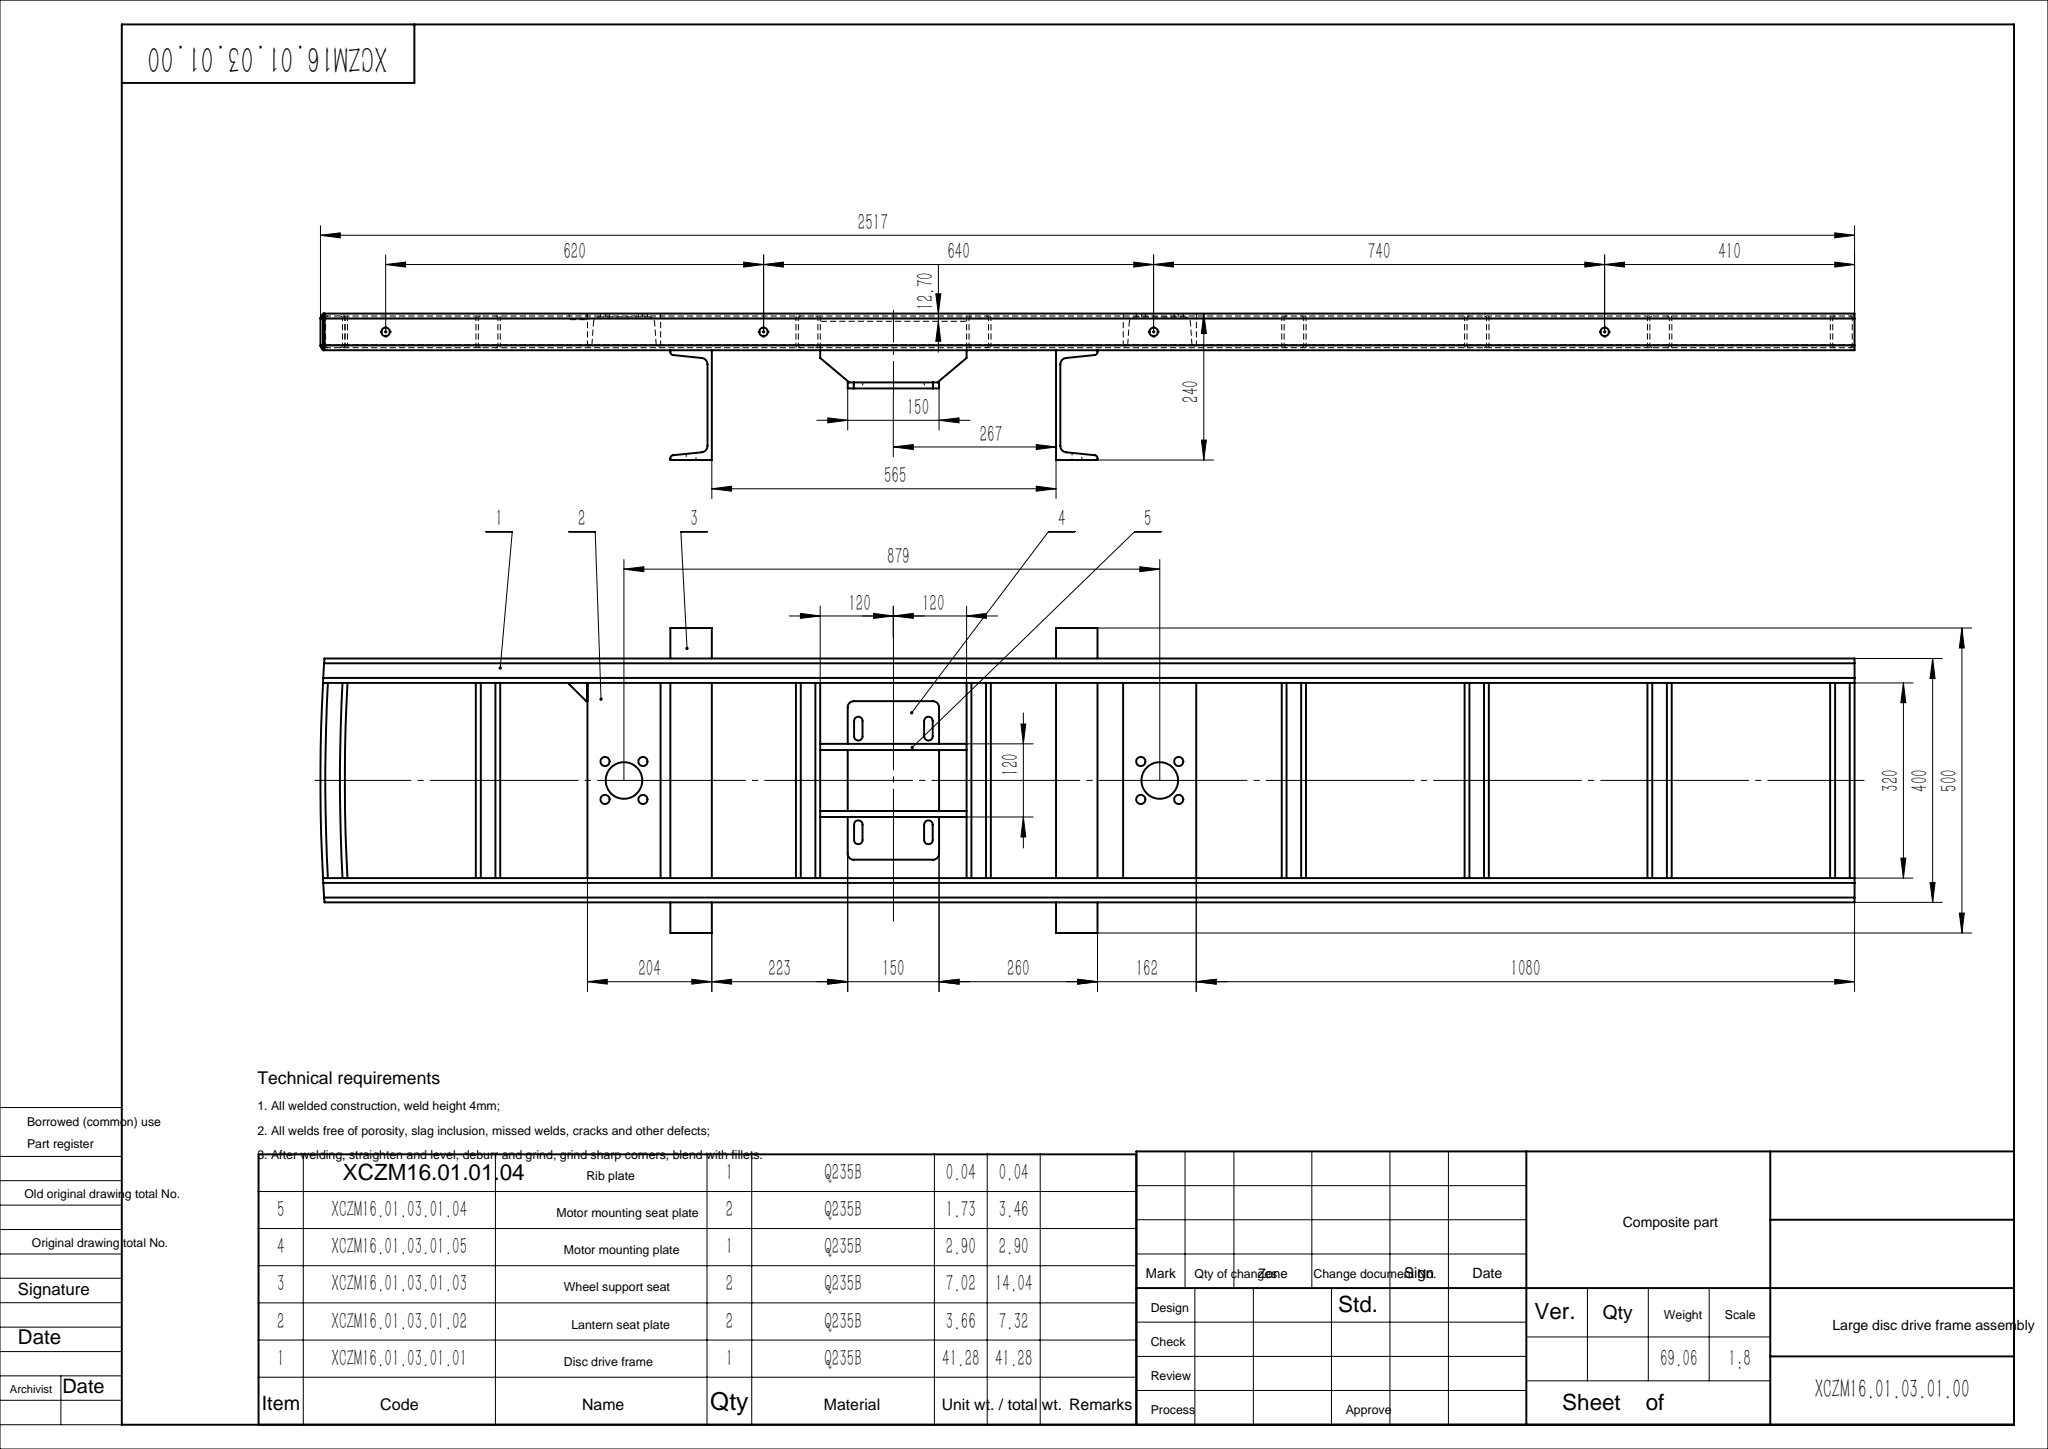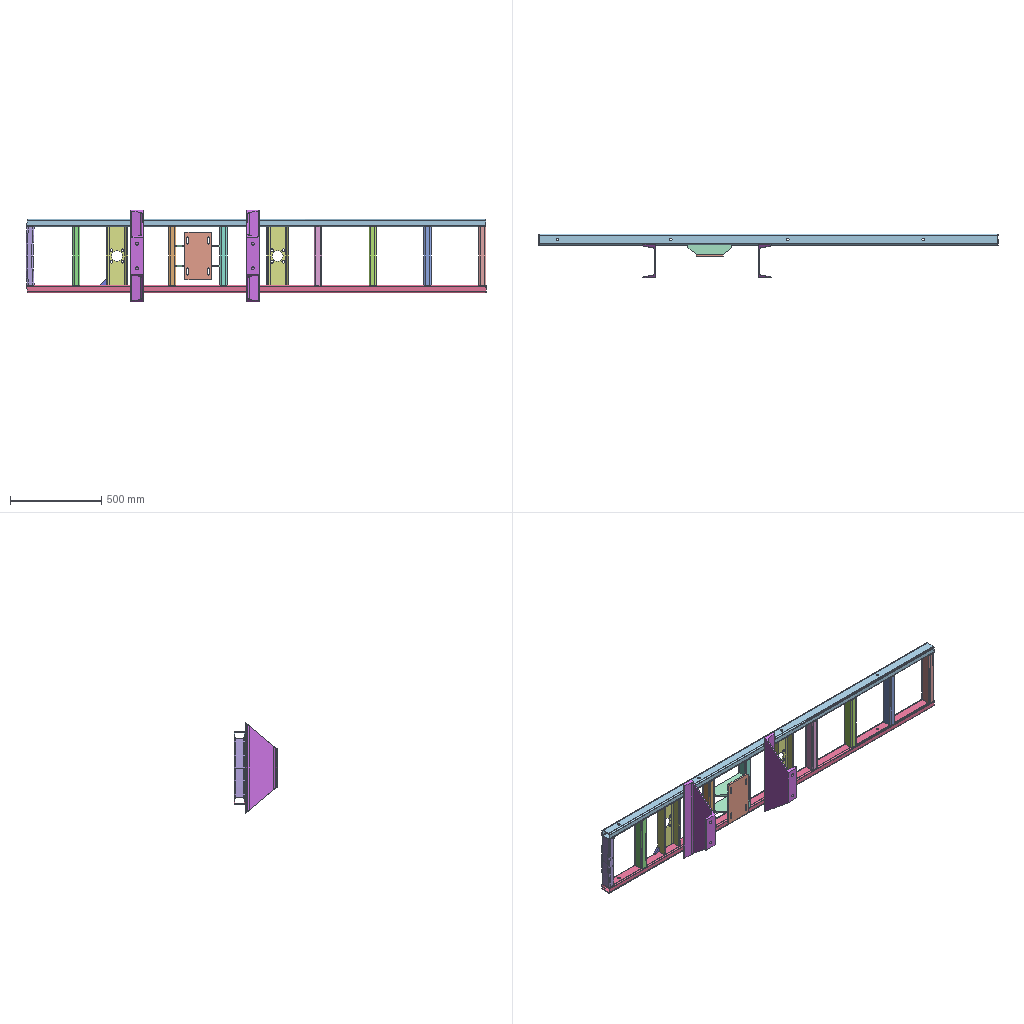Assembly | SolidWorks | 6 different items | 9 placed | box 2517 x 240 x 500 mm
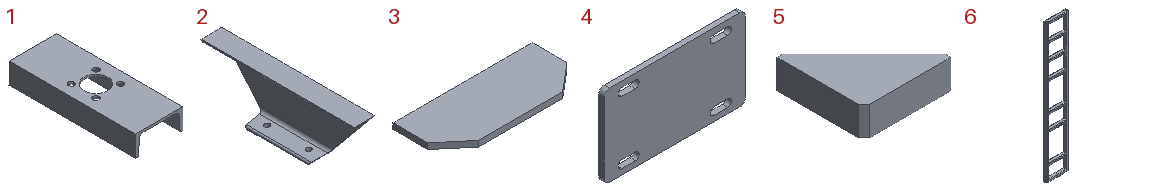Parts list (item | quantity | size | volume | features):
1 | x2 | 120 x 320 x 53 mm | 466744 mm3 | features ICE 1, WeldMemberFeat 1, WeldmentFeature 1
2 | x2 | 68 x 500 x 180 mm | 894795 mm3 | features HoleWzd 1, ICE 1, WeldMemberFeat 1, WeldmentFeature 1
3 | x2 | 240 x 100 x 10 mm | 221000 mm3 | features Extrusion 1
4 | x1 | 260 x 10 x 150 mm | 368984 mm3 | features Extrusion 1
5 | x1 | 30 x 30 x 10 mm | 5060 mm3 | features Chamfer 1, Extrusion 1
6 | x1 | 400 x 60 x 2517 mm | 5259030 mm3 | features HoleWzd 1, WeldMemberFeat 1, WeldmentFeature 1
Mates (type | each side: item.copy, entity, surface, feature):
Coincident | 6.1 face plane Cold-Formed Rectangular Hollow Section(gb t6728-2002) 60×40×4(1) | assembly plane | 2 times
Coincident | 6.1 plane | assembly plane
Coincident | 6.1 face plane Cold-Formed Rectangular Hollow Section(gb t6728-2002) 60×40×4(1) | 1.1 face plane Channel Steel 12(1) | 2 times
DistanceDim | 1.1 face plane Channel Steel 12(1) | 6.1 face plane Cold-Formed Rectangular Hollow Section(gb t6728-2002) 60×40×4(1)
Coincident | 1.1 face plane Channel Steel 12(1) | 1.2 face plane Channel Steel 12(1) | 2 times
DistanceDim | 1.2 face plane Channel Steel 12(1) | 6.1 face plane Cold-Formed Rectangular Hollow Section(gb t6728-2002) 60×40×4(1)
DistanceDim | 2.1 face plane Hot-Rolled Channel Steel(gb t707-1988) 18A-XXXXXXXXXXXXXXX528V9(2) | 6.1 face plane Cold-Formed Rectangular Hollow Section(gb t6728-2002) 60×40×4(1)
Coincident | 2.1 face plane Hot-Rolled Channel Steel(gb t707-1988) 18A-XXXXXXXXXXXXXXX528V9(2) | 2.2 face plane Hot-Rolled Channel Steel(gb t707-1988) 18A-XXXXXXXXXXXXXXX528V9(2)
DistanceDim | 2.1 face plane Hot-Rolled Channel Steel(gb t707-1988) 18A-XXXXXXXXXXXXXXX528V9(2) | 2.2 face plane Hot-Rolled Channel Steel(gb t707-1988) 18A-XXXXXXXXXXXXXXX528V9(2)
Coincident | 6.1 face plane Cold-Formed Rectangular Hollow Section(gb t6728-2002) 60×40×4(1) | 2.1 face plane Hot-Rolled Channel Steel(gb t707-1988) 18A-XXXXXXXXXXXXXXX528V9(2)
Coincident | 2.1 edge | 2.2 edge
Symmetric | 2.1 edge | 2.1 edge | assembly plane
Coincident | 6.1 face plane Cold-Formed Rectangular Hollow Section(gb t6728-2002) 60×40×4(1) | 3.1 face plane Boss-Extrude 1
Coincident | 3.1 face plane Boss-Extrude 1 | 3.2 face plane Boss-Extrude 1 | 2 times
Coincident | 4.1 face plane Boss-Extrude 1 | 3.1 face plane Boss-Extrude 1
DistanceDim | 6.1 face plane Cold-Formed Rectangular Hollow Section(gb t6728-2002) 60×40×4(1) | 3.1 face plane Boss-Extrude 1
DistanceDim | 3.1 face plane Boss-Extrude 1 | 3.2 face plane Boss-Extrude 1
Width | 6.1 face plane Cold-Formed Rectangular Hollow Section(gb t6728-2002) 60×40×4(1) | 6.1 face plane Cold-Formed Rectangular Hollow Section(gb t6728-2002) 60×40×4(1) | 3.2 face plane Boss-Extrude 1 | 3.1 face plane Boss-Extrude 1
Width | 4.1 face plane Boss-Extrude 1 | 4.1 face plane Boss-Extrude 1 | 3.1 face plane Boss-Extrude 1 | 3.2 face plane Boss-Extrude 1
Width | 3.1 face plane Boss-Extrude 1 | 3.2 face plane Boss-Extrude 1 | 4.1 face plane Boss-Extrude 1 | 4.1 face plane Boss-Extrude 1
Coincident | 1.1 face plane Channel Steel 12(1) | 5.1 face plane Boss-Extrude 1 | 2 times
Coincident | 6.1 face plane Cold-Formed Rectangular Hollow Section(gb t6728-2002) 60×40×4(1) | 5.1 face plane Boss-Extrude 1